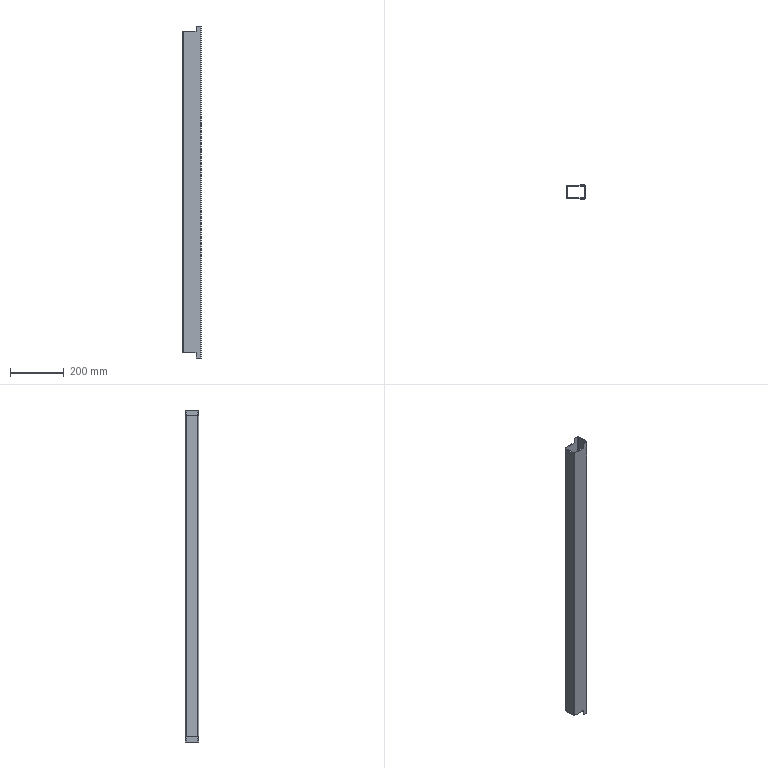Part | SolidWorks | features BaseBody 1 | 1 solid | 24 faces | box 70 x 50 x 1236 mm | volume 549298 mm3 | plane 16 | cylinder 8 | commonest cylinder face diameters 4 x4 8 x4
STEP:
#1=CARTESIAN_POINT('',(15.,23.,598.));
#2=VERTEX_POINT('',#1);
#3=CARTESIAN_POINT('',(15.,23.,618.));
#4=VERTEX_POINT('',#3);
#5=CARTESIAN_POINT('',(15.,23.,618.));
#6=DIRECTION('',(0.,0.,1.));
#7=VECTOR('',#6,1000.);
#8=LINE('',#5,#7);
#9=EDGE_CURVE('',#2,#4,#8,.T.);
#10=ORIENTED_EDGE('',*,*,#9,.T.);
#11=CARTESIAN_POINT('',(15.,25.,618.));
#12=VERTEX_POINT('',#11);
#13=CARTESIAN_POINT('',(15.,25.,618.));
#14=DIRECTION('',(0.,-1.,0.));
#15=VECTOR('',#14,1000.);
#16=LINE('',#13,#15);
#17=EDGE_CURVE('',#12,#4,#16,.T.);
#18=ORIENTED_EDGE('',*,*,#17,.F.);
#19=CARTESIAN_POINT('',(15.,25.,598.));
#20=VERTEX_POINT('',#19);
#21=CARTESIAN_POINT('',(15.,25.,618.));
#22=DIRECTION('',(0.,0.,1.));
#23=VECTOR('',#22,1000.);
#24=LINE('',#21,#23);
#25=EDGE_CURVE('',#20,#12,#24,.T.);
#26=ORIENTED_EDGE('',*,*,#25,.F.);
#27=CARTESIAN_POINT('',(15.,25.,598.));
#28=DIRECTION('',(0.,-1.,0.));
#29=VECTOR('',#28,1000.);
#30=LINE('',#27,#29);
#31=EDGE_CURVE('',#20,#2,#30,.T.);
#32=ORIENTED_EDGE('',*,*,#31,.T.);
#33=EDGE_LOOP('',(#10,#18,#26,#32));
#34=FACE_OUTER_BOUND('',#33,.T.);
#35=CARTESIAN_POINT('',(15.,25.,618.));
#36=DIRECTION('',(1.,0.,0.));
#37=DIRECTION('',(0.,0.,1.));
#38=AXIS2_PLACEMENT_3D('',#35,#36,#37);
#39=PLANE('',#38);
#40=ADVANCED_FACE('',(#34),#39,.F.);
#41=CARTESIAN_POINT('',(-31.,-25.,598.));
#42=VERTEX_POINT('',#41);
#43=CARTESIAN_POINT('',(15.,-25.,598.));
#44=VERTEX_POINT('',#43);
#45=CARTESIAN_POINT('',(-35.,-25.,598.));
#46=DIRECTION('',(1.,0.,0.));
#47=VECTOR('',#46,1000.);
#48=LINE('',#45,#47);
#49=EDGE_CURVE('',#42,#44,#48,.T.);
#50=ORIENTED_EDGE('',*,*,#49,.T.);
#51=CARTESIAN_POINT('',(15.,-23.,598.));
#52=VERTEX_POINT('',#51);
#53=CARTESIAN_POINT('',(15.,25.,598.));
#54=DIRECTION('',(0.,-1.,0.));
#55=VECTOR('',#54,1000.);
#56=LINE('',#53,#55);
#57=EDGE_CURVE('',#52,#44,#56,.T.);
#58=ORIENTED_EDGE('',*,*,#57,.F.);
#59=CARTESIAN_POINT('',(-31.,-23.,598.));
#60=VERTEX_POINT('',#59);
#61=CARTESIAN_POINT('',(-31.,-23.,598.));
#62=DIRECTION('',(-1.,0.,0.));
#63=VECTOR('',#62,1000.);
#64=LINE('',#61,#63);
#65=EDGE_CURVE('',#52,#60,#64,.T.);
#66=ORIENTED_EDGE('',*,*,#65,.T.);
#67=CARTESIAN_POINT('',(-33.,-21.,598.));
#68=VERTEX_POINT('',#67);
#69=CARTESIAN_POINT('',(-31.,-21.,598.));
#70=DIRECTION('',(0.,0.,-1.));
#71=DIRECTION('',(-1.,0.,0.));
#72=AXIS2_PLACEMENT_3D('',#69,#70,#71);
#73=CIRCLE('',#72,2.);
#74=EDGE_CURVE('',#60,#68,#73,.T.);
#75=ORIENTED_EDGE('',*,*,#74,.T.);
#76=CARTESIAN_POINT('',(-33.,21.,598.));
#77=VERTEX_POINT('',#76);
#78=CARTESIAN_POINT('',(-33.,21.,598.));
#79=DIRECTION('',(0.,1.,0.));
#80=VECTOR('',#79,1000.);
#81=LINE('',#78,#80);
#82=EDGE_CURVE('',#68,#77,#81,.T.);
#83=ORIENTED_EDGE('',*,*,#82,.T.);
#84=CARTESIAN_POINT('',(-31.,23.,598.));
#85=VERTEX_POINT('',#84);
#86=CARTESIAN_POINT('',(-31.,21.,598.));
#87=DIRECTION('',(0.,0.,-1.));
#88=DIRECTION('',(-1.,0.,0.));
#89=AXIS2_PLACEMENT_3D('',#86,#87,#88);
#90=CIRCLE('',#89,2.);
#91=EDGE_CURVE('',#77,#85,#90,.T.);
#92=ORIENTED_EDGE('',*,*,#91,.T.);
#93=CARTESIAN_POINT('',(-31.,23.,598.));
#94=DIRECTION('',(1.,0.,0.));
#95=VECTOR('',#94,1000.);
#96=LINE('',#93,#95);
#97=EDGE_CURVE('',#85,#2,#96,.T.);
#98=ORIENTED_EDGE('',*,*,#97,.T.);
#99=ORIENTED_EDGE('',*,*,#31,.F.);
#100=CARTESIAN_POINT('',(-31.,25.,598.));
#101=VERTEX_POINT('',#100);
#102=CARTESIAN_POINT('',(-35.,25.,598.));
#103=DIRECTION('',(1.,0.,0.));
#104=VECTOR('',#103,1000.);
#105=LINE('',#102,#104);
#106=EDGE_CURVE('',#101,#20,#105,.T.);
#107=ORIENTED_EDGE('',*,*,#106,.F.);
#108=CARTESIAN_POINT('',(-35.,21.,598.));
#109=VERTEX_POINT('',#108);
#110=CARTESIAN_POINT('',(-31.,21.,598.));
#111=DIRECTION('',(0.,0.,-1.));
#112=DIRECTION('',(-1.,0.,0.));
#113=AXIS2_PLACEMENT_3D('',#110,#111,#112);
#114=CIRCLE('',#113,4.);
#115=EDGE_CURVE('',#109,#101,#114,.T.);
#116=ORIENTED_EDGE('',*,*,#115,.F.);
#117=CARTESIAN_POINT('',(-35.,-21.,598.));
#118=VERTEX_POINT('',#117);
#119=CARTESIAN_POINT('',(-35.,25.,598.));
#120=DIRECTION('',(0.,-1.,0.));
#121=VECTOR('',#120,1000.);
#122=LINE('',#119,#121);
#123=EDGE_CURVE('',#109,#118,#122,.T.);
#124=ORIENTED_EDGE('',*,*,#123,.T.);
#125=CARTESIAN_POINT('',(-31.,-21.,598.));
#126=DIRECTION('',(0.,0.,-1.));
#127=DIRECTION('',(-1.,0.,0.));
#128=AXIS2_PLACEMENT_3D('',#125,#126,#127);
#129=CIRCLE('',#128,4.);
#130=EDGE_CURVE('',#42,#118,#129,.T.);
#131=ORIENTED_EDGE('',*,*,#130,.F.);
#132=EDGE_LOOP('',(#50,#58,#66,#75,#83,#92,#98,#99,#107,#116,#124,#131));
#133=FACE_OUTER_BOUND('',#132,.T.);
#134=CARTESIAN_POINT('',(-35.,25.,598.));
#135=DIRECTION('',(0.,0.,-1.));
#136=DIRECTION('',(0.,-1.,0.));
#137=AXIS2_PLACEMENT_3D('',#134,#135,#136);
#138=PLANE('',#137);
#139=ADVANCED_FACE('',(#133),#138,.F.);
#140=CARTESIAN_POINT('',(15.,-23.,618.));
#141=VERTEX_POINT('',#140);
#142=CARTESIAN_POINT('',(15.,-23.,618.));
#143=DIRECTION('',(0.,0.,-1.));
#144=VECTOR('',#143,1000.);
#145=LINE('',#142,#144);
#146=EDGE_CURVE('',#141,#52,#145,.T.);
#147=ORIENTED_EDGE('',*,*,#146,.T.);
#148=ORIENTED_EDGE('',*,*,#57,.T.);
#149=CARTESIAN_POINT('',(15.,-25.,618.));
#150=VERTEX_POINT('',#149);
#151=CARTESIAN_POINT('',(15.,-25.,618.));
#152=DIRECTION('',(0.,0.,1.));
#153=VECTOR('',#152,1000.);
#154=LINE('',#151,#153);
#155=EDGE_CURVE('',#44,#150,#154,.T.);
#156=ORIENTED_EDGE('',*,*,#155,.T.);
#157=CARTESIAN_POINT('',(15.,25.,618.));
#158=DIRECTION('',(0.,-1.,0.));
#159=VECTOR('',#158,1000.);
#160=LINE('',#157,#159);
#161=EDGE_CURVE('',#141,#150,#160,.T.);
#162=ORIENTED_EDGE('',*,*,#161,.F.);
#163=EDGE_LOOP('',(#147,#148,#156,#162));
#164=FACE_OUTER_BOUND('',#163,.T.);
#165=CARTESIAN_POINT('',(15.,25.,618.));
#166=DIRECTION('',(1.,0.,0.));
#167=DIRECTION('',(0.,0.,1.));
#168=AXIS2_PLACEMENT_3D('',#165,#166,#167);
#169=PLANE('',#168);
#170=ADVANCED_FACE('',(#164),#169,.F.);
#171=CARTESIAN_POINT('',(15.,23.,-618.));
#172=VERTEX_POINT('',#171);
#173=CARTESIAN_POINT('',(15.,23.,-598.));
#174=VERTEX_POINT('',#173);
#175=CARTESIAN_POINT('',(15.,23.,618.));
#176=DIRECTION('',(0.,0.,1.));
#177=VECTOR('',#176,1000.);
#178=LINE('',#175,#177);
#179=EDGE_CURVE('',#172,#174,#178,.T.);
#180=ORIENTED_EDGE('',*,*,#179,.T.);
#181=CARTESIAN_POINT('',(15.,25.,-598.));
#182=VERTEX_POINT('',#181);
#183=CARTESIAN_POINT('',(15.,25.,-598.));
#184=DIRECTION('',(0.,-1.,0.));
#185=VECTOR('',#184,1000.);
#186=LINE('',#183,#185);
#187=EDGE_CURVE('',#182,#174,#186,.T.);
#188=ORIENTED_EDGE('',*,*,#187,.F.);
#189=CARTESIAN_POINT('',(15.,25.,-618.));
#190=VERTEX_POINT('',#189);
#191=CARTESIAN_POINT('',(15.,25.,-618.));
#192=DIRECTION('',(0.,0.,1.));
#193=VECTOR('',#192,1000.);
#194=LINE('',#191,#193);
#195=EDGE_CURVE('',#190,#182,#194,.T.);
#196=ORIENTED_EDGE('',*,*,#195,.F.);
#197=CARTESIAN_POINT('',(15.,25.,-618.));
#198=DIRECTION('',(0.,-1.,0.));
#199=VECTOR('',#198,1000.);
#200=LINE('',#197,#199);
#201=EDGE_CURVE('',#190,#172,#200,.T.);
#202=ORIENTED_EDGE('',*,*,#201,.T.);
#203=EDGE_LOOP('',(#180,#188,#196,#202));
#204=FACE_OUTER_BOUND('',#203,.T.);
#205=CARTESIAN_POINT('',(15.,25.,-618.));
#206=DIRECTION('',(1.,0.,0.));
#207=DIRECTION('',(0.,0.,-1.));
#208=AXIS2_PLACEMENT_3D('',#205,#206,#207);
#209=PLANE('',#208);
#210=ADVANCED_FACE('',(#204),#209,.F.);
#211=CARTESIAN_POINT('',(-35.,21.,-598.));
#212=VERTEX_POINT('',#211);
#213=CARTESIAN_POINT('',(-35.,-21.,-598.));
#214=VERTEX_POINT('',#213);
#215=CARTESIAN_POINT('',(-35.,25.,-598.));
#216=DIRECTION('',(0.,-1.,0.));
#217=VECTOR('',#216,1000.);
#218=LINE('',#215,#217);
#219=EDGE_CURVE('',#212,#214,#218,.T.);
#220=ORIENTED_EDGE('',*,*,#219,.F.);
#221=CARTESIAN_POINT('',(-31.,25.,-598.));
#222=VERTEX_POINT('',#221);
#223=CARTESIAN_POINT('',(-31.,21.,-598.));
#224=DIRECTION('',(0.,0.,1.));
#225=DIRECTION('',(1.,0.,0.));
#226=AXIS2_PLACEMENT_3D('',#223,#224,#225);
#227=CIRCLE('',#226,4.);
#228=EDGE_CURVE('',#222,#212,#227,.T.);
#229=ORIENTED_EDGE('',*,*,#228,.F.);
#230=CARTESIAN_POINT('',(-35.,25.,-598.));
#231=DIRECTION('',(-1.,0.,0.));
#232=VECTOR('',#231,1000.);
#233=LINE('',#230,#232);
#234=EDGE_CURVE('',#182,#222,#233,.T.);
#235=ORIENTED_EDGE('',*,*,#234,.F.);
#236=ORIENTED_EDGE('',*,*,#187,.T.);
#237=CARTESIAN_POINT('',(-31.,23.,-598.));
#238=VERTEX_POINT('',#237);
#239=CARTESIAN_POINT('',(-31.,23.,-598.));
#240=DIRECTION('',(-1.,0.,0.));
#241=VECTOR('',#240,1000.);
#242=LINE('',#239,#241);
#243=EDGE_CURVE('',#174,#238,#242,.T.);
#244=ORIENTED_EDGE('',*,*,#243,.T.);
#245=CARTESIAN_POINT('',(-33.,21.,-598.));
#246=VERTEX_POINT('',#245);
#247=CARTESIAN_POINT('',(-31.,21.,-598.));
#248=DIRECTION('',(0.,0.,1.));
#249=DIRECTION('',(1.,0.,0.));
#250=AXIS2_PLACEMENT_3D('',#247,#248,#249);
#251=CIRCLE('',#250,2.);
#252=EDGE_CURVE('',#238,#246,#251,.T.);
#253=ORIENTED_EDGE('',*,*,#252,.T.);
#254=CARTESIAN_POINT('',(-33.,-21.,-598.));
#255=VERTEX_POINT('',#254);
#256=CARTESIAN_POINT('',(-33.,21.,-598.));
#257=DIRECTION('',(0.,-1.,0.));
#258=VECTOR('',#257,1000.);
#259=LINE('',#256,#258);
#260=EDGE_CURVE('',#246,#255,#259,.T.);
#261=ORIENTED_EDGE('',*,*,#260,.T.);
#262=CARTESIAN_POINT('',(-31.,-23.,-598.));
#263=VERTEX_POINT('',#262);
#264=CARTESIAN_POINT('',(-31.,-21.,-598.));
#265=DIRECTION('',(0.,0.,1.));
#266=DIRECTION('',(1.,0.,0.));
#267=AXIS2_PLACEMENT_3D('',#264,#265,#266);
#268=CIRCLE('',#267,2.);
#269=EDGE_CURVE('',#255,#263,#268,.T.);
#270=ORIENTED_EDGE('',*,*,#269,.T.);
#271=CARTESIAN_POINT('',(15.,-23.,-598.));
#272=VERTEX_POINT('',#271);
#273=CARTESIAN_POINT('',(-31.,-23.,-598.));
#274=DIRECTION('',(1.,0.,0.));
#275=VECTOR('',#274,1000.);
#276=LINE('',#273,#275);
#277=EDGE_CURVE('',#263,#272,#276,.T.);
#278=ORIENTED_EDGE('',*,*,#277,.T.);
#279=CARTESIAN_POINT('',(15.,-25.,-598.));
#280=VERTEX_POINT('',#279);
#281=CARTESIAN_POINT('',(15.,25.,-598.));
#282=DIRECTION('',(0.,-1.,0.));
#283=VECTOR('',#282,1000.);
#284=LINE('',#281,#283);
#285=EDGE_CURVE('',#272,#280,#284,.T.);
#286=ORIENTED_EDGE('',*,*,#285,.T.);
#287=CARTESIAN_POINT('',(-31.,-25.,-598.));
#288=VERTEX_POINT('',#287);
#289=CARTESIAN_POINT('',(-35.,-25.,-598.));
#290=DIRECTION('',(-1.,0.,0.));
#291=VECTOR('',#290,1000.);
#292=LINE('',#289,#291);
#293=EDGE_CURVE('',#280,#288,#292,.T.);
#294=ORIENTED_EDGE('',*,*,#293,.T.);
#295=CARTESIAN_POINT('',(-31.,-21.,-598.));
#296=DIRECTION('',(0.,0.,1.));
#297=DIRECTION('',(1.,0.,0.));
#298=AXIS2_PLACEMENT_3D('',#295,#296,#297);
#299=CIRCLE('',#298,4.);
#300=EDGE_CURVE('',#214,#288,#299,.T.);
#301=ORIENTED_EDGE('',*,*,#300,.F.);
#302=EDGE_LOOP('',(#220,#229,#235,#236,#244,#253,#261,#270,#278,#286,#294,#301));
#303=FACE_OUTER_BOUND('',#302,.T.);
#304=CARTESIAN_POINT('',(-35.,25.,-598.));
#305=DIRECTION('',(0.,0.,1.));
#306=DIRECTION('',(1.,0.,0.));
#307=AXIS2_PLACEMENT_3D('',#304,#305,#306);
#308=PLANE('',#307);
#309=ADVANCED_FACE('',(#303),#308,.F.);
#310=CARTESIAN_POINT('',(15.,-23.,-618.));
#311=VERTEX_POINT('',#310);
#312=CARTESIAN_POINT('',(15.,-23.,618.));
#313=DIRECTION('',(0.,0.,-1.));
#314=VECTOR('',#313,1000.);
#315=LINE('',#312,#314);
#316=EDGE_CURVE('',#272,#311,#315,.T.);
#317=ORIENTED_EDGE('',*,*,#316,.T.);
#318=CARTESIAN_POINT('',(15.,-25.,-618.));
#319=VERTEX_POINT('',#318);
#320=CARTESIAN_POINT('',(15.,25.,-618.));
#321=DIRECTION('',(0.,-1.,0.));
#322=VECTOR('',#321,1000.);
#323=LINE('',#320,#322);
#324=EDGE_CURVE('',#311,#319,#323,.T.);
#325=ORIENTED_EDGE('',*,*,#324,.T.);
#326=CARTESIAN_POINT('',(15.,-25.,-618.));
#327=DIRECTION('',(0.,0.,1.));
#328=VECTOR('',#327,1000.);
#329=LINE('',#326,#328);
#330=EDGE_CURVE('',#319,#280,#329,.T.);
#331=ORIENTED_EDGE('',*,*,#330,.T.);
#332=ORIENTED_EDGE('',*,*,#285,.F.);
#333=EDGE_LOOP('',(#317,#325,#331,#332));
#334=FACE_OUTER_BOUND('',#333,.T.);
#335=CARTESIAN_POINT('',(15.,25.,-618.));
#336=DIRECTION('',(1.,0.,0.));
#337=DIRECTION('',(0.,0.,-1.));
#338=AXIS2_PLACEMENT_3D('',#335,#336,#337);
#339=PLANE('',#338);
#340=ADVANCED_FACE('',(#334),#339,.F.);
#341=ORIENTED_EDGE('',*,*,#82,.F.);
#342=CARTESIAN_POINT('',(-33.,-21.,618.));
#343=DIRECTION('',(0.,0.,-1.));
#344=VECTOR('',#343,1000.);
#345=LINE('',#342,#344);
#346=EDGE_CURVE('',#68,#255,#345,.T.);
#347=ORIENTED_EDGE('',*,*,#346,.T.);
#348=ORIENTED_EDGE('',*,*,#260,.F.);
#349=CARTESIAN_POINT('',(-33.,21.,618.));
#350=DIRECTION('',(0.,0.,-1.));
#351=VECTOR('',#350,1000.);
#352=LINE('',#349,#351);
#353=EDGE_CURVE('',#77,#246,#352,.T.);
#354=ORIENTED_EDGE('',*,*,#353,.F.);
#355=EDGE_LOOP('',(#341,#347,#348,#354));
#356=FACE_OUTER_BOUND('',#355,.T.);
#357=CARTESIAN_POINT('',(-33.,21.,618.));
#358=DIRECTION('',(1.,0.,0.));
#359=DIRECTION('',(0.,1.,0.));
#360=AXIS2_PLACEMENT_3D('',#357,#358,#359);
#361=PLANE('',#360);
#362=ADVANCED_FACE('',(#356),#361,.T.);
#363=ORIENTED_EDGE('',*,*,#91,.F.);
#364=ORIENTED_EDGE('',*,*,#353,.T.);
#365=ORIENTED_EDGE('',*,*,#252,.F.);
#366=CARTESIAN_POINT('',(-31.,23.,618.));
#367=DIRECTION('',(0.,0.,-1.));
#368=VECTOR('',#367,1000.);
#369=LINE('',#366,#368);
#370=EDGE_CURVE('',#85,#238,#369,.T.);
#371=ORIENTED_EDGE('',*,*,#370,.F.);
#372=EDGE_LOOP('',(#363,#364,#365,#371));
#373=FACE_OUTER_BOUND('',#372,.T.);
#374=CARTESIAN_POINT('',(-31.,21.,618.));
#375=DIRECTION('',(0.,0.,-1.));
#376=DIRECTION('',(-1.,0.,0.));
#377=AXIS2_PLACEMENT_3D('',#374,#375,#376);
#378=CYLINDRICAL_SURFACE('',#377,2.);
#379=ADVANCED_FACE('',(#373),#378,.F.);
#380=ORIENTED_EDGE('',*,*,#9,.F.);
#381=ORIENTED_EDGE('',*,*,#97,.F.);
#382=ORIENTED_EDGE('',*,*,#370,.T.);
#383=ORIENTED_EDGE('',*,*,#243,.F.);
#384=ORIENTED_EDGE('',*,*,#179,.F.);
#385=CARTESIAN_POINT('',(31.,23.,-618.));
#386=VERTEX_POINT('',#385);
#387=CARTESIAN_POINT('',(-31.,23.,-618.));
#388=DIRECTION('',(-1.,0.,0.));
#389=VECTOR('',#388,1000.);
#390=LINE('',#387,#389);
#391=EDGE_CURVE('',#386,#172,#390,.T.);
#392=ORIENTED_EDGE('',*,*,#391,.F.);
#393=CARTESIAN_POINT('',(31.,23.,618.));
#394=VERTEX_POINT('',#393);
#395=CARTESIAN_POINT('',(31.,23.,618.));
#396=DIRECTION('',(0.,0.,-1.));
#397=VECTOR('',#396,1000.);
#398=LINE('',#395,#397);
#399=EDGE_CURVE('',#394,#386,#398,.T.);
#400=ORIENTED_EDGE('',*,*,#399,.F.);
#401=CARTESIAN_POINT('',(-31.,23.,618.));
#402=DIRECTION('',(-1.,0.,0.));
#403=VECTOR('',#402,1000.);
#404=LINE('',#401,#403);
#405=EDGE_CURVE('',#394,#4,#404,.T.);
#406=ORIENTED_EDGE('',*,*,#405,.T.);
#407=EDGE_LOOP('',(#380,#381,#382,#383,#384,#392,#400,#406));
#408=FACE_OUTER_BOUND('',#407,.T.);
#409=CARTESIAN_POINT('',(-31.,23.,618.));
#410=DIRECTION('',(0.,-1.,0.));
#411=DIRECTION('',(0.,0.,-1.));
#412=AXIS2_PLACEMENT_3D('',#409,#410,#411);
#413=PLANE('',#412);
#414=ADVANCED_FACE('',(#408),#413,.T.);
#415=CARTESIAN_POINT('',(33.,21.,-618.));
#416=VERTEX_POINT('',#415);
#417=CARTESIAN_POINT('',(31.,21.,-618.));
#418=DIRECTION('',(0.,0.,1.));
#419=DIRECTION('',(1.,0.,0.));
#420=AXIS2_PLACEMENT_3D('',#417,#418,#419);
#421=CIRCLE('',#420,2.);
#422=EDGE_CURVE('',#416,#386,#421,.T.);
#423=ORIENTED_EDGE('',*,*,#422,.F.);
#424=CARTESIAN_POINT('',(33.,21.,618.));
#425=VERTEX_POINT('',#424);
#426=CARTESIAN_POINT('',(33.,21.,618.));
#427=DIRECTION('',(0.,0.,-1.));
#428=VECTOR('',#427,1000.);
#429=LINE('',#426,#428);
#430=EDGE_CURVE('',#425,#416,#429,.T.);
#431=ORIENTED_EDGE('',*,*,#430,.F.);
#432=CARTESIAN_POINT('',(31.,21.,618.));
#433=DIRECTION('',(0.,0.,1.));
#434=DIRECTION('',(1.,0.,0.));
#435=AXIS2_PLACEMENT_3D('',#432,#433,#434);
#436=CIRCLE('',#435,2.);
#437=EDGE_CURVE('',#425,#394,#436,.T.);
#438=ORIENTED_EDGE('',*,*,#437,.T.);
#439=ORIENTED_EDGE('',*,*,#399,.T.);
#440=EDGE_LOOP('',(#423,#431,#438,#439));
#441=FACE_OUTER_BOUND('',#440,.T.);
#442=CARTESIAN_POINT('',(31.,21.,618.));
#443=DIRECTION('',(0.,0.,-1.));
#444=DIRECTION('',(-1.,0.,0.));
#445=AXIS2_PLACEMENT_3D('',#442,#443,#444);
#446=CYLINDRICAL_SURFACE('',#445,2.);
#447=ADVANCED_FACE('',(#441),#446,.F.);
#448=CARTESIAN_POINT('',(33.,-21.,-618.));
#449=VERTEX_POINT('',#448);
#450=CARTESIAN_POINT('',(33.,21.,-618.));
#451=DIRECTION('',(0.,1.,0.));
#452=VECTOR('',#451,1000.);
#453=LINE('',#450,#452);
#454=EDGE_CURVE('',#449,#416,#453,.T.);
#455=ORIENTED_EDGE('',*,*,#454,.F.);
#456=CARTESIAN_POINT('',(33.,-21.,618.));
#457=VERTEX_POINT('',#456);
#458=CARTESIAN_POINT('',(33.,-21.,618.));
#459=DIRECTION('',(0.,0.,-1.));
#460=VECTOR('',#459,1000.);
#461=LINE('',#458,#460);
#462=EDGE_CURVE('',#457,#449,#461,.T.);
#463=ORIENTED_EDGE('',*,*,#462,.F.);
#464=CARTESIAN_POINT('',(33.,21.,618.));
#465=DIRECTION('',(0.,1.,0.));
#466=VECTOR('',#465,1000.);
#467=LINE('',#464,#466);
#468=EDGE_CURVE('',#457,#425,#467,.T.);
#469=ORIENTED_EDGE('',*,*,#468,.T.);
#470=ORIENTED_EDGE('',*,*,#430,.T.);
#471=EDGE_LOOP('',(#455,#463,#469,#470));
#472=FACE_OUTER_BOUND('',#471,.T.);
#473=CARTESIAN_POINT('',(33.,21.,618.));
#474=DIRECTION('',(-1.,0.,0.));
#475=DIRECTION('',(0.,1.,0.));
#476=AXIS2_PLACEMENT_3D('',#473,#474,#475);
#477=PLANE('',#476);
#478=ADVANCED_FACE('',(#472),#477,.T.);
#479=CARTESIAN_POINT('',(31.,-23.,-618.));
#480=VERTEX_POINT('',#479);
#481=CARTESIAN_POINT('',(31.,-21.,-618.));
#482=DIRECTION('',(0.,0.,1.));
#483=DIRECTION('',(1.,0.,0.));
#484=AXIS2_PLACEMENT_3D('',#481,#482,#483);
#485=CIRCLE('',#484,2.);
#486=EDGE_CURVE('',#480,#449,#485,.T.);
#487=ORIENTED_EDGE('',*,*,#486,.F.);
#488=CARTESIAN_POINT('',(31.,-23.,618.));
#489=VERTEX_POINT('',#488);
#490=CARTESIAN_POINT('',(31.,-23.,618.));
#491=DIRECTION('',(0.,0.,-1.));
#492=VECTOR('',#491,1000.);
#493=LINE('',#490,#492);
#494=EDGE_CURVE('',#489,#480,#493,.T.);
#495=ORIENTED_EDGE('',*,*,#494,.F.);
#496=CARTESIAN_POINT('',(31.,-21.,618.));
#497=DIRECTION('',(0.,0.,1.));
#498=DIRECTION('',(1.,0.,0.));
#499=AXIS2_PLACEMENT_3D('',#496,#497,#498);
#500=CIRCLE('',#499,2.);
#501=EDGE_CURVE('',#489,#457,#500,.T.);
#502=ORIENTED_EDGE('',*,*,#501,.T.);
#503=ORIENTED_EDGE('',*,*,#462,.T.);
#504=EDGE_LOOP('',(#487,#495,#502,#503));
#505=FACE_OUTER_BOUND('',#504,.T.);
#506=CARTESIAN_POINT('',(31.,-21.,618.));
#507=DIRECTION('',(0.,0.,-1.));
#508=DIRECTION('',(-1.,0.,0.));
#509=AXIS2_PLACEMENT_3D('',#506,#507,#508);
#510=CYLINDRICAL_SURFACE('',#509,2.);
#511=ADVANCED_FACE('',(#505),#510,.F.);
#512=ORIENTED_EDGE('',*,*,#146,.F.);
#513=CARTESIAN_POINT('',(-31.,-23.,618.));
#514=DIRECTION('',(1.,0.,0.));
#515=VECTOR('',#514,1000.);
#516=LINE('',#513,#515);
#517=EDGE_CURVE('',#141,#489,#516,.T.);
#518=ORIENTED_EDGE('',*,*,#517,.T.);
#519=ORIENTED_EDGE('',*,*,#494,.T.);
#520=CARTESIAN_POINT('',(-31.,-23.,-618.));
#521=DIRECTION('',(1.,0.,0.));
#522=VECTOR('',#521,1000.);
#523=LINE('',#520,#522);
#524=EDGE_CURVE('',#311,#480,#523,.T.);
#525=ORIENTED_EDGE('',*,*,#524,.F.);
#526=ORIENTED_EDGE('',*,*,#316,.F.);
#527=ORIENTED_EDGE('',*,*,#277,.F.);
#528=CARTESIAN_POINT('',(-31.,-23.,618.));
#529=DIRECTION('',(0.,0.,-1.));
#530=VECTOR('',#529,1000.);
#531=LINE('',#528,#530);
#532=EDGE_CURVE('',#60,#263,#531,.T.);
#533=ORIENTED_EDGE('',*,*,#532,.F.);
#534=ORIENTED_EDGE('',*,*,#65,.F.);
#535=EDGE_LOOP('',(#512,#518,#519,#525,#526,#527,#533,#534));
#536=FACE_OUTER_BOUND('',#535,.T.);
#537=CARTESIAN_POINT('',(-31.,-23.,618.));
#538=DIRECTION('',(0.,1.,0.));
#539=DIRECTION('',(1.,0.,0.));
#540=AXIS2_PLACEMENT_3D('',#537,#538,#539);
#541=PLANE('',#540);
#542=ADVANCED_FACE('',(#536),#541,.T.);
#543=ORIENTED_EDGE('',*,*,#74,.F.);
#544=ORIENTED_EDGE('',*,*,#532,.T.);
#545=ORIENTED_EDGE('',*,*,#269,.F.);
#546=ORIENTED_EDGE('',*,*,#346,.F.);
#547=EDGE_LOOP('',(#543,#544,#545,#546));
#548=FACE_OUTER_BOUND('',#547,.T.);
#549=CARTESIAN_POINT('',(-31.,-21.,618.));
#550=DIRECTION('',(0.,0.,-1.));
#551=DIRECTION('',(-1.,0.,0.));
#552=AXIS2_PLACEMENT_3D('',#549,#550,#551);
#553=CYLINDRICAL_SURFACE('',#552,2.);
#554=ADVANCED_FACE('',(#548),#553,.F.);
#555=CARTESIAN_POINT('',(-35.,-21.,618.));
#556=DIRECTION('',(0.,0.,-1.));
#557=VECTOR('',#556,1000.);
#558=LINE('',#555,#557);
#559=EDGE_CURVE('',#118,#214,#558,.T.);
#560=ORIENTED_EDGE('',*,*,#559,.F.);
#561=ORIENTED_EDGE('',*,*,#123,.F.);
#562=CARTESIAN_POINT('',(-35.,21.,618.));
#563=DIRECTION('',(0.,0.,-1.));
#564=VECTOR('',#563,1000.);
#565=LINE('',#562,#564);
#566=EDGE_CURVE('',#109,#212,#565,.T.);
#567=ORIENTED_EDGE('',*,*,#566,.T.);
#568=ORIENTED_EDGE('',*,*,#219,.T.);
#569=EDGE_LOOP('',(#560,#561,#567,#568));
#570=FACE_OUTER_BOUND('',#569,.T.);
#571=CARTESIAN_POINT('',(-35.,21.,618.));
#572=DIRECTION('',(1.,0.,0.));
#573=DIRECTION('',(0.,1.,0.));
#574=AXIS2_PLACEMENT_3D('',#571,#572,#573);
#575=PLANE('',#574);
#576=ADVANCED_FACE('',(#570),#575,.F.);
#577=ORIENTED_EDGE('',*,*,#566,.F.);
#578=ORIENTED_EDGE('',*,*,#115,.T.);
#579=CARTESIAN_POINT('',(-31.,25.,618.));
#580=DIRECTION('',(0.,0.,-1.));
#581=VECTOR('',#580,1000.);
#582=LINE('',#579,#581);
#583=EDGE_CURVE('',#101,#222,#582,.T.);
#584=ORIENTED_EDGE('',*,*,#583,.T.);
#585=ORIENTED_EDGE('',*,*,#228,.T.);
#586=EDGE_LOOP('',(#577,#578,#584,#585));
#587=FACE_OUTER_BOUND('',#586,.T.);
#588=CARTESIAN_POINT('',(-31.,21.,618.));
#589=DIRECTION('',(0.,0.,-1.));
#590=DIRECTION('',(-1.,0.,0.));
#591=AXIS2_PLACEMENT_3D('',#588,#589,#590);
#592=CYLINDRICAL_SURFACE('',#591,4.);
#593=ADVANCED_FACE('',(#587),#592,.T.);
#594=ORIENTED_EDGE('',*,*,#106,.T.);
#595=ORIENTED_EDGE('',*,*,#25,.T.);
#596=CARTESIAN_POINT('',(31.,25.,618.));
#597=VERTEX_POINT('',#596);
#598=CARTESIAN_POINT('',(-31.,25.,618.));
#599=DIRECTION('',(-1.,0.,0.));
#600=VECTOR('',#599,1000.);
#601=LINE('',#598,#600);
#602=EDGE_CURVE('',#597,#12,#601,.T.);
#603=ORIENTED_EDGE('',*,*,#602,.F.);
#604=CARTESIAN_POINT('',(31.,25.,-618.));
#605=VERTEX_POINT('',#604);
#606=CARTESIAN_POINT('',(31.,25.,618.));
#607=DIRECTION('',(0.,0.,-1.));
#608=VECTOR('',#607,1000.);
#609=LINE('',#606,#608);
#610=EDGE_CURVE('',#597,#605,#609,.T.);
#611=ORIENTED_EDGE('',*,*,#610,.T.);
#612=CARTESIAN_POINT('',(-31.,25.,-618.));
#613=DIRECTION('',(-1.,0.,0.));
#614=VECTOR('',#613,1000.);
#615=LINE('',#612,#614);
#616=EDGE_CURVE('',#605,#190,#615,.T.);
#617=ORIENTED_EDGE('',*,*,#616,.T.);
#618=ORIENTED_EDGE('',*,*,#195,.T.);
#619=ORIENTED_EDGE('',*,*,#234,.T.);
#620=ORIENTED_EDGE('',*,*,#583,.F.);
#621=EDGE_LOOP('',(#594,#595,#603,#611,#617,#618,#619,#620));
#622=FACE_OUTER_BOUND('',#621,.T.);
#623=CARTESIAN_POINT('',(-31.,25.,618.));
#624=DIRECTION('',(0.,-1.,0.));
#625=DIRECTION('',(0.,0.,-1.));
#626=AXIS2_PLACEMENT_3D('',#623,#624,#625);
#627=PLANE('',#626);
#628=ADVANCED_FACE('',(#622),#627,.F.);
#629=CARTESIAN_POINT('',(35.,21.,-618.));
#630=VERTEX_POINT('',#629);
#631=CARTESIAN_POINT('',(31.,21.,-618.));
#632=DIRECTION('',(0.,0.,1.));
#633=DIRECTION('',(-1.,0.,0.));
#634=AXIS2_PLACEMENT_3D('',#631,#632,#633);
#635=CIRCLE('',#634,4.);
#636=EDGE_CURVE('',#630,#605,#635,.T.);
#637=ORIENTED_EDGE('',*,*,#636,.T.);
#638=ORIENTED_EDGE('',*,*,#610,.F.);
#639=CARTESIAN_POINT('',(35.,21.,618.));
#640=VERTEX_POINT('',#639);
#641=CARTESIAN_POINT('',(31.,21.,618.));
#642=DIRECTION('',(0.,0.,1.));
#643=DIRECTION('',(-1.,0.,0.));
#644=AXIS2_PLACEMENT_3D('',#641,#642,#643);
#645=CIRCLE('',#644,4.);
#646=EDGE_CURVE('',#640,#597,#645,.T.);
#647=ORIENTED_EDGE('',*,*,#646,.F.);
#648=CARTESIAN_POINT('',(35.,21.,618.));
#649=DIRECTION('',(0.,0.,-1.));
#650=VECTOR('',#649,1000.);
#651=LINE('',#648,#650);
#652=EDGE_CURVE('',#640,#630,#651,.T.);
#653=ORIENTED_EDGE('',*,*,#652,.T.);
#654=EDGE_LOOP('',(#637,#638,#647,#653));
#655=FACE_OUTER_BOUND('',#654,.T.);
#656=CARTESIAN_POINT('',(31.,21.,618.));
#657=DIRECTION('',(0.,0.,-1.));
#658=DIRECTION('',(-1.,0.,0.));
#659=AXIS2_PLACEMENT_3D('',#656,#657,#658);
#660=CYLINDRICAL_SURFACE('',#659,4.);
#661=ADVANCED_FACE('',(#655),#660,.T.);
#662=CARTESIAN_POINT('',(35.,-21.,-618.));
#663=VERTEX_POINT('',#662);
#664=CARTESIAN_POINT('',(35.,21.,-618.));
#665=DIRECTION('',(0.,1.,0.));
#666=VECTOR('',#665,1000.);
#667=LINE('',#664,#666);
#668=EDGE_CURVE('',#663,#630,#667,.T.);
#669=ORIENTED_EDGE('',*,*,#668,.T.);
#670=ORIENTED_EDGE('',*,*,#652,.F.);
#671=CARTESIAN_POINT('',(35.,-21.,618.));
#672=VERTEX_POINT('',#671);
#673=CARTESIAN_POINT('',(35.,21.,618.));
#674=DIRECTION('',(0.,1.,0.));
#675=VECTOR('',#674,1000.);
#676=LINE('',#673,#675);
#677=EDGE_CURVE('',#672,#640,#676,.T.);
#678=ORIENTED_EDGE('',*,*,#677,.F.);
#679=CARTESIAN_POINT('',(35.,-21.,618.));
#680=DIRECTION('',(0.,0.,-1.));
#681=VECTOR('',#680,1000.);
#682=LINE('',#679,#681);
#683=EDGE_CURVE('',#672,#663,#682,.T.);
#684=ORIENTED_EDGE('',*,*,#683,.T.);
#685=EDGE_LOOP('',(#669,#670,#678,#684));
#686=FACE_OUTER_BOUND('',#685,.T.);
#687=CARTESIAN_POINT('',(35.,21.,618.));
#688=DIRECTION('',(-1.,0.,0.));
#689=DIRECTION('',(0.,1.,0.));
#690=AXIS2_PLACEMENT_3D('',#687,#688,#689);
#691=PLANE('',#690);
#692=ADVANCED_FACE('',(#686),#691,.F.);
#693=CARTESIAN_POINT('',(31.,-25.,-618.));
#694=VERTEX_POINT('',#693);
#695=CARTESIAN_POINT('',(31.,-21.,-618.));
#696=DIRECTION('',(0.,0.,1.));
#697=DIRECTION('',(1.,0.,0.));
#698=AXIS2_PLACEMENT_3D('',#695,#696,#697);
#699=CIRCLE('',#698,4.);
#700=EDGE_CURVE('',#694,#663,#699,.T.);
#701=ORIENTED_EDGE('',*,*,#700,.T.);
#702=ORIENTED_EDGE('',*,*,#683,.F.);
#703=CARTESIAN_POINT('',(31.,-25.,618.));
#704=VERTEX_POINT('',#703);
#705=CARTESIAN_POINT('',(31.,-21.,618.));
#706=DIRECTION('',(0.,0.,1.));
#707=DIRECTION('',(1.,0.,0.));
#708=AXIS2_PLACEMENT_3D('',#705,#706,#707);
#709=CIRCLE('',#708,4.);
#710=EDGE_CURVE('',#704,#672,#709,.T.);
#711=ORIENTED_EDGE('',*,*,#710,.F.);
#712=CARTESIAN_POINT('',(31.,-25.,618.));
#713=DIRECTION('',(0.,0.,-1.));
#714=VECTOR('',#713,1000.);
#715=LINE('',#712,#714);
#716=EDGE_CURVE('',#704,#694,#715,.T.);
#717=ORIENTED_EDGE('',*,*,#716,.T.);
#718=EDGE_LOOP('',(#701,#702,#711,#717));
#719=FACE_OUTER_BOUND('',#718,.T.);
#720=CARTESIAN_POINT('',(31.,-21.,618.));
#721=DIRECTION('',(0.,0.,-1.));
#722=DIRECTION('',(-1.,0.,0.));
#723=AXIS2_PLACEMENT_3D('',#720,#721,#722);
#724=CYLINDRICAL_SURFACE('',#723,4.);
#725=ADVANCED_FACE('',(#719),#724,.T.);
#726=CARTESIAN_POINT('',(-31.,-25.,618.));
#727=DIRECTION('',(1.,0.,0.));
#728=VECTOR('',#727,1000.);
#729=LINE('',#726,#728);
#730=EDGE_CURVE('',#150,#704,#729,.T.);
#731=ORIENTED_EDGE('',*,*,#730,.F.);
#732=ORIENTED_EDGE('',*,*,#155,.F.);
#733=ORIENTED_EDGE('',*,*,#49,.F.);
#734=CARTESIAN_POINT('',(-31.,-25.,618.));
#735=DIRECTION('',(0.,0.,-1.));
#736=VECTOR('',#735,1000.);
#737=LINE('',#734,#736);
#738=EDGE_CURVE('',#42,#288,#737,.T.);
#739=ORIENTED_EDGE('',*,*,#738,.T.);
#740=ORIENTED_EDGE('',*,*,#293,.F.);
#741=ORIENTED_EDGE('',*,*,#330,.F.);
#742=CARTESIAN_POINT('',(-31.,-25.,-618.));
#743=DIRECTION('',(1.,0.,0.));
#744=VECTOR('',#743,1000.);
#745=LINE('',#742,#744);
#746=EDGE_CURVE('',#319,#694,#745,.T.);
#747=ORIENTED_EDGE('',*,*,#746,.T.);
#748=ORIENTED_EDGE('',*,*,#716,.F.);
#749=EDGE_LOOP('',(#731,#732,#733,#739,#740,#741,#747,#748));
#750=FACE_OUTER_BOUND('',#749,.T.);
#751=CARTESIAN_POINT('',(-31.,-25.,618.));
#752=DIRECTION('',(0.,1.,0.));
#753=DIRECTION('',(1.,0.,0.));
#754=AXIS2_PLACEMENT_3D('',#751,#752,#753);
#755=PLANE('',#754);
#756=ADVANCED_FACE('',(#750),#755,.F.);
#757=ORIENTED_EDGE('',*,*,#738,.F.);
#758=ORIENTED_EDGE('',*,*,#130,.T.);
#759=ORIENTED_EDGE('',*,*,#559,.T.);
#760=ORIENTED_EDGE('',*,*,#300,.T.);
#761=EDGE_LOOP('',(#757,#758,#759,#760));
#762=FACE_OUTER_BOUND('',#761,.T.);
#763=CARTESIAN_POINT('',(-31.,-21.,618.));
#764=DIRECTION('',(0.,0.,-1.));
#765=DIRECTION('',(-1.,0.,0.));
#766=AXIS2_PLACEMENT_3D('',#763,#764,#765);
#767=CYLINDRICAL_SURFACE('',#766,4.);
#768=ADVANCED_FACE('',(#762),#767,.T.);
#769=ORIENTED_EDGE('',*,*,#746,.F.);
#770=ORIENTED_EDGE('',*,*,#324,.F.);
#771=ORIENTED_EDGE('',*,*,#524,.T.);
#772=ORIENTED_EDGE('',*,*,#486,.T.);
#773=ORIENTED_EDGE('',*,*,#454,.T.);
#774=ORIENTED_EDGE('',*,*,#422,.T.);
#775=ORIENTED_EDGE('',*,*,#391,.T.);
#776=ORIENTED_EDGE('',*,*,#201,.F.);
#777=ORIENTED_EDGE('',*,*,#616,.F.);
#778=ORIENTED_EDGE('',*,*,#636,.F.);
#779=ORIENTED_EDGE('',*,*,#668,.F.);
#780=ORIENTED_EDGE('',*,*,#700,.F.);
#781=EDGE_LOOP('',(#769,#770,#771,#772,#773,#774,#775,#776,#777,#778,#779,#780));
#782=FACE_OUTER_BOUND('',#781,.T.);
#783=CARTESIAN_POINT('',(-31.,-21.,-618.));
#784=DIRECTION('',(0.,0.,1.));
#785=DIRECTION('',(1.,0.,0.));
#786=AXIS2_PLACEMENT_3D('',#783,#784,#785);
#787=PLANE('',#786);
#788=ADVANCED_FACE('',(#782),#787,.F.);
#789=ORIENTED_EDGE('',*,*,#161,.T.);
#790=ORIENTED_EDGE('',*,*,#730,.T.);
#791=ORIENTED_EDGE('',*,*,#710,.T.);
#792=ORIENTED_EDGE('',*,*,#677,.T.);
#793=ORIENTED_EDGE('',*,*,#646,.T.);
#794=ORIENTED_EDGE('',*,*,#602,.T.);
#795=ORIENTED_EDGE('',*,*,#17,.T.);
#796=ORIENTED_EDGE('',*,*,#405,.F.);
#797=ORIENTED_EDGE('',*,*,#437,.F.);
#798=ORIENTED_EDGE('',*,*,#468,.F.);
#799=ORIENTED_EDGE('',*,*,#501,.F.);
#800=ORIENTED_EDGE('',*,*,#517,.F.);
#801=EDGE_LOOP('',(#789,#790,#791,#792,#793,#794,#795,#796,#797,#798,#799,#800));
#802=FACE_OUTER_BOUND('',#801,.T.);
#803=CARTESIAN_POINT('',(-31.,-21.,618.));
#804=DIRECTION('',(0.,0.,1.));
#805=DIRECTION('',(1.,0.,0.));
#806=AXIS2_PLACEMENT_3D('',#803,#804,#805);
#807=PLANE('',#806);
#808=ADVANCED_FACE('',(#802),#807,.T.);
#809=CLOSED_SHELL('',(#40,#139,#170,#210,#309,#340,#362,#379,#414,#447,#478,#511,#542,#554,#576,#593,#628,#661,#692,#725,#756,#768,#788,#808));
#810=MANIFOLD_SOLID_BREP('',#809);
#811=CARTESIAN_POINT('',(0.,0.,0.));
#812=DIRECTION('',(0.,0.,1.));
#813=DIRECTION('',(1.,0.,0.));
#814=AXIS2_PLACEMENT_3D('',#811,#812,#813);
#815=(LENGTH_UNIT()NAMED_UNIT(*)SI_UNIT(.MILLI.,.METRE.));
#816=UNCERTAINTY_MEASURE_WITH_UNIT(LENGTH_MEASURE(0.00001),#815,'','');
#817=(NAMED_UNIT(*)PLANE_ANGLE_UNIT()SI_UNIT($,.RADIAN.));
#818=(NAMED_UNIT(*)SI_UNIT($,.STERADIAN.)SOLID_ANGLE_UNIT());
#819=(GEOMETRIC_REPRESENTATION_CONTEXT(3)GLOBAL_UNCERTAINTY_ASSIGNED_CONTEXT((#816))GLOBAL_UNIT_ASSIGNED_CONTEXT((#815,#817,#818))REPRESENTATION_CONTEXT('',''));
#820=ADVANCED_BREP_SHAPE_REPRESENTATION('',(#810,#814),#819);